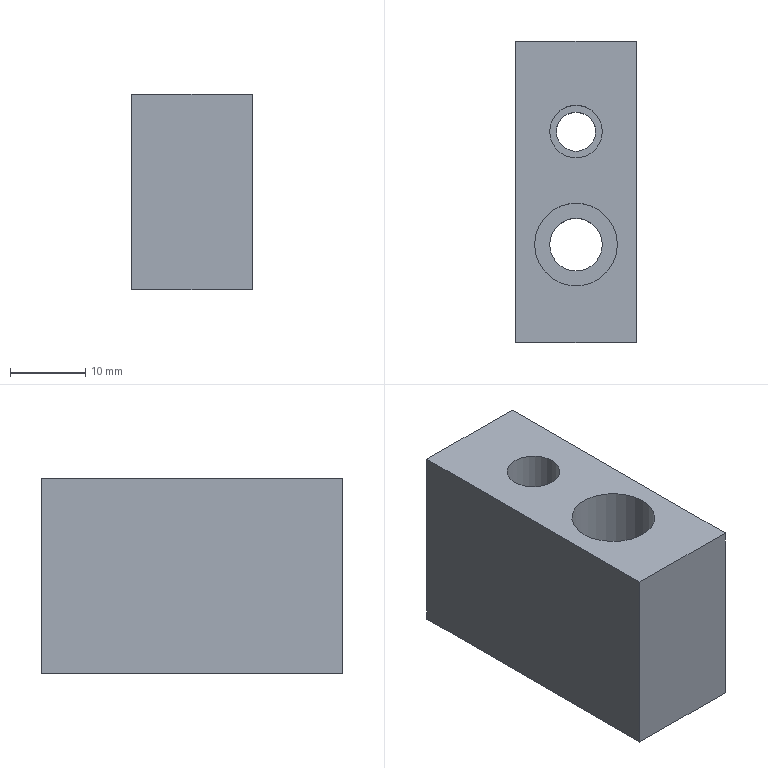Part | NX | features solid 2 | 1 solid | 83 faces | box 16 x 40 x 26 mm | volume 14526 mm3 | plane 65 | spline 14 | cylinder 4 | commonest cylinder face diameters 7 x2 5.2 x1 11 x1